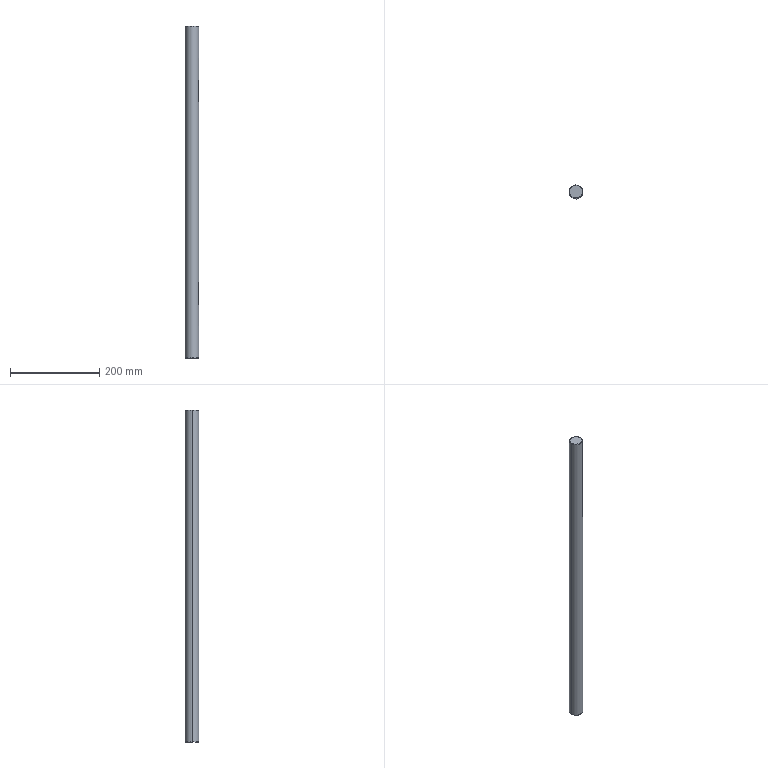Part | STEP file | 1 solid | 20 faces | box 30 x 30 x 742 mm | volume 521298 mm3 | cylinder 8 | plane 8 | spline 4 | commonest cylinder face diameters 8 x6 30 x2